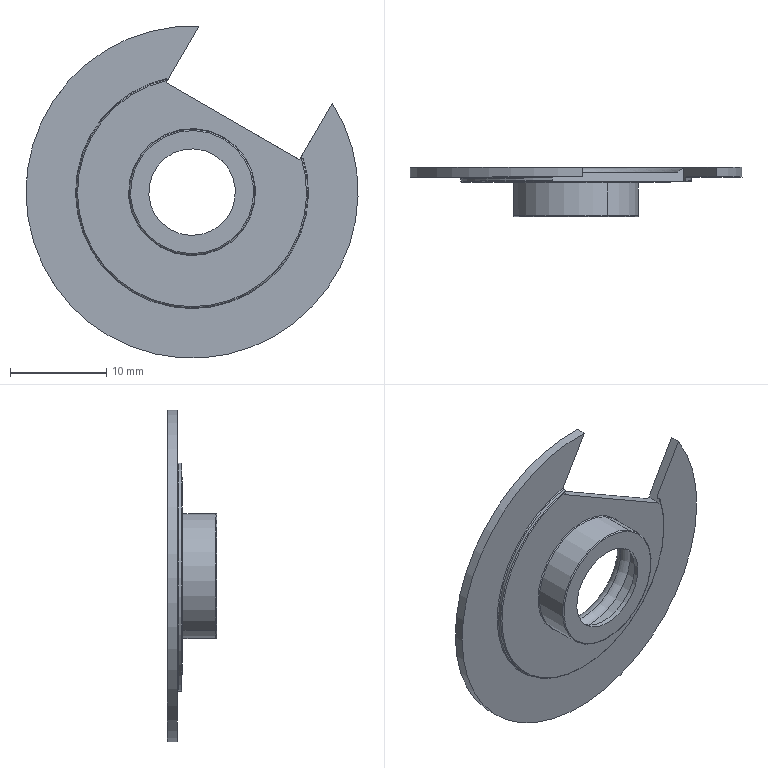Part | SolidWorks | features BaseBody 1 | 1 solid | 31 faces | box 34.501 x 5.123 x 34.5 mm | volume 825.126 mm3 | torus 14 | plane 9 | cylinder 8 | commonest cylinder face diameters 9 x2 12 x2 13 x2 24 x1 34.5 x1
STEP:
#1=CARTESIAN_POINT('',(344.717,378.167,111.682));
#2=VERTEX_POINT('',#1);
#3=CARTESIAN_POINT('',(345.266,379.267,112.635));
#4=VERTEX_POINT('',#3);
#5=CARTESIAN_POINT('',(345.267,378.167,112.635));
#6=DIRECTION('',(0.866,0.0008313,-0.5));
#7=DIRECTION('',(-0.5,0.,-0.866));
#8=AXIS2_PLACEMENT_3D('',#5,#6,#7);
#9=CIRCLE('',#8,1.1);
#10=EDGE_CURVE('',#2,#4,#9,.T.);
#11=ORIENTED_EDGE('',*,*,#10,.F.);
#12=CARTESIAN_POINT('',(339.217,378.161,102.156));
#13=VERTEX_POINT('',#12);
#14=CARTESIAN_POINT('',(341.967,378.164,106.919));
#15=DIRECTION('',(0.0009599,-1.,0.));
#16=DIRECTION('',(1.,0.0009599,0.));
#17=AXIS2_PLACEMENT_3D('',#14,#15,#16);
#18=CIRCLE('',#17,5.5);
#19=EDGE_CURVE('',#2,#13,#18,.T.);
#20=ORIENTED_EDGE('',*,*,#19,.T.);
#21=CARTESIAN_POINT('',(338.666,379.261,101.203));
#22=VERTEX_POINT('',#21);
#23=CARTESIAN_POINT('',(338.667,378.161,101.203));
#24=DIRECTION('',(-0.866,-0.0008313,0.5));
#25=DIRECTION('',(0.5,0.,0.866));
#26=AXIS2_PLACEMENT_3D('',#23,#24,#25);
#27=CIRCLE('',#26,1.1);
#28=EDGE_CURVE('',#13,#22,#27,.T.);
#29=ORIENTED_EDGE('',*,*,#28,.T.);
#30=CARTESIAN_POINT('',(341.966,379.264,106.919));
#31=DIRECTION('',(0.0009599,-1.,0.));
#32=DIRECTION('',(-0.5,-0.0004799,-0.866));
#33=AXIS2_PLACEMENT_3D('',#30,#31,#32);
#34=CIRCLE('',#33,6.6);
#35=EDGE_CURVE('',#4,#22,#34,.T.);
#36=ORIENTED_EDGE('',*,*,#35,.F.);
#37=EDGE_LOOP('',(#11,#20,#29,#36));
#38=FACE_OUTER_BOUND('',#37,.T.);
#39=CARTESIAN_POINT('',(341.967,378.164,106.919));
#40=DIRECTION('',(0.0009599,-1.,0.));
#41=DIRECTION('',(-0.5,-0.0004799,-0.866));
#42=AXIS2_PLACEMENT_3D('',#39,#40,#41);
#43=TOROIDAL_SURFACE('',#42,6.6,1.1);
#44=ADVANCED_FACE('',(#38),#43,.T.);
#45=ORIENTED_EDGE('',*,*,#28,.F.);
#46=CARTESIAN_POINT('',(341.967,378.164,106.919));
#47=DIRECTION('',(0.0009599,-1.,0.));
#48=DIRECTION('',(1.,0.0009599,0.));
#49=AXIS2_PLACEMENT_3D('',#46,#47,#48);
#50=CIRCLE('',#49,5.5);
#51=EDGE_CURVE('',#13,#2,#50,.T.);
#52=ORIENTED_EDGE('',*,*,#51,.T.);
#53=ORIENTED_EDGE('',*,*,#10,.T.);
#54=CARTESIAN_POINT('',(341.966,379.264,106.919));
#55=DIRECTION('',(0.0009599,-1.,0.));
#56=DIRECTION('',(-0.5,-0.0004799,-0.866));
#57=AXIS2_PLACEMENT_3D('',#54,#55,#56);
#58=CIRCLE('',#57,6.6);
#59=EDGE_CURVE('',#22,#4,#58,.T.);
#60=ORIENTED_EDGE('',*,*,#59,.F.);
#61=EDGE_LOOP('',(#45,#52,#53,#60));
#62=FACE_OUTER_BOUND('',#61,.T.);
#63=CARTESIAN_POINT('',(341.967,378.164,106.919));
#64=DIRECTION('',(0.0009599,-1.,0.));
#65=DIRECTION('',(-0.5,-0.0004799,-0.866));
#66=AXIS2_PLACEMENT_3D('',#63,#64,#65);
#67=TOROIDAL_SURFACE('',#66,6.6,1.1);
#68=ADVANCED_FACE('',(#62),#67,.T.);
#69=CARTESIAN_POINT('',(338.717,378.161,101.29));
#70=VERTEX_POINT('',#69);
#71=CARTESIAN_POINT('',(345.217,378.167,112.548));
#72=VERTEX_POINT('',#71);
#73=CARTESIAN_POINT('',(341.967,378.164,106.919));
#74=DIRECTION('',(-0.0009599,1.,0.));
#75=DIRECTION('',(-0.5,-0.0004799,-0.866));
#76=AXIS2_PLACEMENT_3D('',#73,#74,#75);
#77=CIRCLE('',#76,6.5);
#78=EDGE_CURVE('',#70,#72,#77,.T.);
#79=ORIENTED_EDGE('',*,*,#78,.T.);
#80=CARTESIAN_POINT('',(345.267,378.267,112.635));
#81=VERTEX_POINT('',#80);
#82=CARTESIAN_POINT('',(345.267,378.167,112.635));
#83=DIRECTION('',(0.866,0.0008313,-0.5));
#84=DIRECTION('',(-0.5,0.,-0.866));
#85=AXIS2_PLACEMENT_3D('',#82,#83,#84);
#86=CIRCLE('',#85,0.1);
#87=EDGE_CURVE('',#72,#81,#86,.T.);
#88=ORIENTED_EDGE('',*,*,#87,.T.);
#89=CARTESIAN_POINT('',(338.667,378.261,101.203));
#90=VERTEX_POINT('',#89);
#91=CARTESIAN_POINT('',(341.967,378.264,106.919));
#92=DIRECTION('',(-0.0009599,1.,0.));
#93=DIRECTION('',(0.5,0.0004799,0.866));
#94=AXIS2_PLACEMENT_3D('',#91,#92,#93);
#95=CIRCLE('',#94,6.6);
#96=EDGE_CURVE('',#90,#81,#95,.T.);
#97=ORIENTED_EDGE('',*,*,#96,.F.);
#98=CARTESIAN_POINT('',(338.667,378.161,101.203));
#99=DIRECTION('',(-0.866,-0.0008313,0.5));
#100=DIRECTION('',(0.5,0.,0.866));
#101=AXIS2_PLACEMENT_3D('',#98,#99,#100);
#102=CIRCLE('',#101,0.1);
#103=EDGE_CURVE('',#70,#90,#102,.T.);
#104=ORIENTED_EDGE('',*,*,#103,.F.);
#105=EDGE_LOOP('',(#79,#88,#97,#104));
#106=FACE_OUTER_BOUND('',#105,.T.);
#107=CARTESIAN_POINT('',(341.967,378.164,106.919));
#108=DIRECTION('',(0.0009599,-1.,0.));
#109=DIRECTION('',(-0.5,-0.0004799,-0.866));
#110=AXIS2_PLACEMENT_3D('',#107,#108,#109);
#111=TOROIDAL_SURFACE('',#110,6.6,0.1);
#112=ADVANCED_FACE('',(#106),#111,.F.);
#113=CARTESIAN_POINT('',(338.72,374.761,101.29));
#114=VERTEX_POINT('',#113);
#115=CARTESIAN_POINT('',(345.22,374.767,112.548));
#116=VERTEX_POINT('',#115);
#117=CARTESIAN_POINT('',(341.97,374.764,106.919));
#118=DIRECTION('',(0.0009599,-1.,0.));
#119=DIRECTION('',(0.5,0.0004799,0.866));
#120=AXIS2_PLACEMENT_3D('',#117,#118,#119);
#121=CIRCLE('',#120,6.5);
#122=EDGE_CURVE('',#114,#116,#121,.T.);
#123=ORIENTED_EDGE('',*,*,#122,.F.);
#124=CARTESIAN_POINT('',(338.72,374.661,101.29));
#125=DIRECTION('',(-0.0009599,1.,0.));
#126=VECTOR('',#125,1000.);
#127=LINE('',#124,#126);
#128=EDGE_CURVE('',#114,#70,#127,.T.);
#129=ORIENTED_EDGE('',*,*,#128,.T.);
#130=CARTESIAN_POINT('',(341.967,378.164,106.919));
#131=DIRECTION('',(-0.0009599,1.,0.));
#132=DIRECTION('',(-0.5,-0.0004799,-0.866));
#133=AXIS2_PLACEMENT_3D('',#130,#131,#132);
#134=CIRCLE('',#133,6.5);
#135=EDGE_CURVE('',#72,#70,#134,.T.);
#136=ORIENTED_EDGE('',*,*,#135,.F.);
#137=CARTESIAN_POINT('',(345.22,374.667,112.548));
#138=DIRECTION('',(-0.0009599,1.,0.));
#139=VECTOR('',#138,1000.);
#140=LINE('',#137,#139);
#141=EDGE_CURVE('',#116,#72,#140,.T.);
#142=ORIENTED_EDGE('',*,*,#141,.F.);
#143=EDGE_LOOP('',(#123,#129,#136,#142));
#144=FACE_OUTER_BOUND('',#143,.T.);
#145=CARTESIAN_POINT('',(341.97,374.664,106.919));
#146=DIRECTION('',(-0.0009599,1.,0.));
#147=DIRECTION('',(0.5,0.0004799,0.866));
#148=AXIS2_PLACEMENT_3D('',#145,#146,#147);
#149=CYLINDRICAL_SURFACE('',#148,6.5);
#150=ADVANCED_FACE('',(#144),#149,.T.);
#151=ORIENTED_EDGE('',*,*,#122,.T.);
#152=CARTESIAN_POINT('',(345.17,374.667,112.462));
#153=VERTEX_POINT('',#152);
#154=CARTESIAN_POINT('',(345.17,374.767,112.462));
#155=DIRECTION('',(0.866,0.0008313,-0.5));
#156=DIRECTION('',(-0.5,0.,-0.866));
#157=AXIS2_PLACEMENT_3D('',#154,#155,#156);
#158=CIRCLE('',#157,0.1);
#159=EDGE_CURVE('',#116,#153,#158,.T.);
#160=ORIENTED_EDGE('',*,*,#159,.T.);
#161=CARTESIAN_POINT('',(338.77,374.661,101.377));
#162=VERTEX_POINT('',#161);
#163=CARTESIAN_POINT('',(341.97,374.664,106.919));
#164=DIRECTION('',(0.0009599,-1.,0.));
#165=DIRECTION('',(-0.5,-0.0004799,-0.866));
#166=AXIS2_PLACEMENT_3D('',#163,#164,#165);
#167=CIRCLE('',#166,6.4);
#168=EDGE_CURVE('',#162,#153,#167,.T.);
#169=ORIENTED_EDGE('',*,*,#168,.F.);
#170=CARTESIAN_POINT('',(338.77,374.761,101.377));
#171=DIRECTION('',(-0.866,-0.0008313,0.5));
#172=DIRECTION('',(0.5,0.,0.866));
#173=AXIS2_PLACEMENT_3D('',#170,#171,#172);
#174=CIRCLE('',#173,0.1);
#175=EDGE_CURVE('',#114,#162,#174,.T.);
#176=ORIENTED_EDGE('',*,*,#175,.F.);
#177=EDGE_LOOP('',(#151,#160,#169,#176));
#178=FACE_OUTER_BOUND('',#177,.T.);
#179=CARTESIAN_POINT('',(341.97,374.764,106.919));
#180=DIRECTION('',(0.0009599,-1.,0.));
#181=DIRECTION('',(-0.5,-0.0004799,-0.866));
#182=AXIS2_PLACEMENT_3D('',#179,#180,#181);
#183=TOROIDAL_SURFACE('',#182,6.4,0.1);
#184=ADVANCED_FACE('',(#178),#183,.T.);
#185=CARTESIAN_POINT('',(344.22,375.166,110.816));
#186=VERTEX_POINT('',#185);
#187=CARTESIAN_POINT('',(339.72,375.162,103.022));
#188=VERTEX_POINT('',#187);
#189=CARTESIAN_POINT('',(341.97,375.164,106.919));
#190=DIRECTION('',(0.0009599,-1.,0.));
#191=DIRECTION('',(-0.5,-0.0004799,-0.866));
#192=AXIS2_PLACEMENT_3D('',#189,#190,#191);
#193=CIRCLE('',#192,4.5);
#194=EDGE_CURVE('',#186,#188,#193,.T.);
#195=ORIENTED_EDGE('',*,*,#194,.F.);
#196=CARTESIAN_POINT('',(344.22,374.666,110.816));
#197=VERTEX_POINT('',#196);
#198=CARTESIAN_POINT('',(344.217,378.266,110.816));
#199=DIRECTION('',(0.0009599,-1.,0.));
#200=VECTOR('',#199,1000.);
#201=LINE('',#198,#200);
#202=EDGE_CURVE('',#186,#197,#201,.T.);
#203=ORIENTED_EDGE('',*,*,#202,.T.);
#204=CARTESIAN_POINT('',(339.72,374.662,103.022));
#205=VERTEX_POINT('',#204);
#206=CARTESIAN_POINT('',(341.97,374.664,106.919));
#207=DIRECTION('',(-0.0009599,1.,0.));
#208=DIRECTION('',(-0.5,-0.0004799,-0.866));
#209=AXIS2_PLACEMENT_3D('',#206,#207,#208);
#210=CIRCLE('',#209,4.5);
#211=EDGE_CURVE('',#205,#197,#210,.T.);
#212=ORIENTED_EDGE('',*,*,#211,.F.);
#213=CARTESIAN_POINT('',(339.717,378.262,103.022));
#214=DIRECTION('',(0.0009599,-1.,0.));
#215=VECTOR('',#214,1000.);
#216=LINE('',#213,#215);
#217=EDGE_CURVE('',#188,#205,#216,.T.);
#218=ORIENTED_EDGE('',*,*,#217,.F.);
#219=EDGE_LOOP('',(#195,#203,#212,#218));
#220=FACE_OUTER_BOUND('',#219,.T.);
#221=CARTESIAN_POINT('',(341.967,378.264,106.919));
#222=DIRECTION('',(0.0009599,-1.,0.));
#223=DIRECTION('',(-0.5,-0.0004799,-0.866));
#224=AXIS2_PLACEMENT_3D('',#221,#222,#223);
#225=CYLINDRICAL_SURFACE('',#224,4.5);
#226=ADVANCED_FACE('',(#220),#225,.F.);
#227=CARTESIAN_POINT('',(338.97,375.161,101.723));
#228=VERTEX_POINT('',#227);
#229=CARTESIAN_POINT('',(344.97,375.167,112.115));
#230=VERTEX_POINT('',#229);
#231=CARTESIAN_POINT('',(341.97,375.164,106.919));
#232=DIRECTION('',(-0.0009599,1.,0.));
#233=DIRECTION('',(0.5,0.0004799,0.866));
#234=AXIS2_PLACEMENT_3D('',#231,#232,#233);
#235=CIRCLE('',#234,6.);
#236=EDGE_CURVE('',#228,#230,#235,.T.);
#237=ORIENTED_EDGE('',*,*,#236,.F.);
#238=CARTESIAN_POINT('',(338.968,377.239,101.723));
#239=VERTEX_POINT('',#238);
#240=CARTESIAN_POINT('',(338.97,374.661,101.723));
#241=DIRECTION('',(-0.0009599,1.,0.));
#242=VECTOR('',#241,1000.);
#243=LINE('',#240,#242);
#244=EDGE_CURVE('',#228,#239,#243,.T.);
#245=ORIENTED_EDGE('',*,*,#244,.T.);
#246=CARTESIAN_POINT('',(344.968,377.245,112.115));
#247=VERTEX_POINT('',#246);
#248=CARTESIAN_POINT('',(341.968,377.242,106.919));
#249=DIRECTION('',(0.0009599,-1.,0.));
#250=DIRECTION('',(0.5,0.0004799,0.866));
#251=AXIS2_PLACEMENT_3D('',#248,#249,#250);
#252=CIRCLE('',#251,6.);
#253=EDGE_CURVE('',#247,#239,#252,.T.);
#254=ORIENTED_EDGE('',*,*,#253,.F.);
#255=CARTESIAN_POINT('',(344.97,374.667,112.115));
#256=DIRECTION('',(-0.0009599,1.,0.));
#257=VECTOR('',#256,1000.);
#258=LINE('',#255,#257);
#259=EDGE_CURVE('',#230,#247,#258,.T.);
#260=ORIENTED_EDGE('',*,*,#259,.F.);
#261=EDGE_LOOP('',(#237,#245,#254,#260));
#262=FACE_OUTER_BOUND('',#261,.T.);
#263=CARTESIAN_POINT('',(341.97,374.664,106.919));
#264=DIRECTION('',(-0.0009599,1.,0.));
#265=DIRECTION('',(0.5,0.0004799,0.866));
#266=AXIS2_PLACEMENT_3D('',#263,#264,#265);
#267=CYLINDRICAL_SURFACE('',#266,6.);
#268=ADVANCED_FACE('',(#262),#267,.F.);
#269=ORIENTED_EDGE('',*,*,#51,.F.);
#270=CARTESIAN_POINT('',(338.667,378.161,101.203));
#271=DIRECTION('',(-0.866,-0.0008313,0.5));
#272=DIRECTION('',(0.5,0.,0.866));
#273=AXIS2_PLACEMENT_3D('',#270,#271,#272);
#274=CIRCLE('',#273,1.1);
#275=EDGE_CURVE('',#239,#13,#274,.T.);
#276=ORIENTED_EDGE('',*,*,#275,.F.);
#277=CARTESIAN_POINT('',(341.968,377.242,106.919));
#278=DIRECTION('',(0.0009599,-1.,0.));
#279=DIRECTION('',(0.5,0.0004799,0.866));
#280=AXIS2_PLACEMENT_3D('',#277,#278,#279);
#281=CIRCLE('',#280,6.);
#282=EDGE_CURVE('',#239,#247,#281,.T.);
#283=ORIENTED_EDGE('',*,*,#282,.T.);
#284=CARTESIAN_POINT('',(345.267,378.167,112.635));
#285=DIRECTION('',(0.866,0.0008313,-0.5));
#286=DIRECTION('',(-0.5,0.,-0.866));
#287=AXIS2_PLACEMENT_3D('',#284,#285,#286);
#288=CIRCLE('',#287,1.1);
#289=EDGE_CURVE('',#247,#2,#288,.T.);
#290=ORIENTED_EDGE('',*,*,#289,.T.);
#291=EDGE_LOOP('',(#269,#276,#283,#290));
#292=FACE_OUTER_BOUND('',#291,.T.);
#293=CARTESIAN_POINT('',(341.967,378.164,106.919));
#294=DIRECTION('',(0.0009599,-1.,0.));
#295=DIRECTION('',(-0.5,-0.0004799,-0.866));
#296=AXIS2_PLACEMENT_3D('',#293,#294,#295);
#297=TOROIDAL_SURFACE('',#296,6.6,1.1);
#298=ADVANCED_FACE('',(#292),#297,.T.);
#299=CARTESIAN_POINT('',(336.377,379.259,97.239));
#300=VERTEX_POINT('',#299);
#301=CARTESIAN_POINT('',(339.929,379.262,117.91));
#302=VERTEX_POINT('',#301);
#303=CARTESIAN_POINT('',(341.966,379.264,106.919));
#304=DIRECTION('',(-0.0009599,1.,0.));
#305=DIRECTION('',(0.9426,0.0009048,0.3338));
#306=AXIS2_PLACEMENT_3D('',#303,#304,#305);
#307=CIRCLE('',#306,11.178);
#308=EDGE_CURVE('',#300,#302,#307,.T.);
#309=ORIENTED_EDGE('',*,*,#308,.F.);
#310=CARTESIAN_POINT('',(335.915,379.758,96.44));
#311=VERTEX_POINT('',#310);
#312=CARTESIAN_POINT('',(335.916,378.658,96.44));
#313=DIRECTION('',(-0.866,-0.0008313,0.5));
#314=DIRECTION('',(0.5,0.,0.866));
#315=AXIS2_PLACEMENT_3D('',#312,#313,#314);
#316=CIRCLE('',#315,1.1);
#317=EDGE_CURVE('',#300,#311,#316,.T.);
#318=ORIENTED_EDGE('',*,*,#317,.T.);
#319=CARTESIAN_POINT('',(339.576,379.762,118.781));
#320=VERTEX_POINT('',#319);
#321=CARTESIAN_POINT('',(341.965,379.764,106.919));
#322=DIRECTION('',(0.0009599,-1.,0.));
#323=DIRECTION('',(-0.1975,-0.0001895,0.9803));
#324=AXIS2_PLACEMENT_3D('',#321,#322,#323);
#325=CIRCLE('',#324,12.1);
#326=EDGE_CURVE('',#320,#311,#325,.T.);
#327=ORIENTED_EDGE('',*,*,#326,.F.);
#328=CARTESIAN_POINT('',(339.287,379.675,118.28));
#329=VERTEX_POINT('',#328);
#330=CARTESIAN_POINT('',(339.576,379.762,118.781));
#331=CARTESIAN_POINT('',(339.478,379.762,118.61));
#332=CARTESIAN_POINT('',(339.381,379.733,118.443));
#333=CARTESIAN_POINT('',(339.287,379.675,118.28));
#334=B_SPLINE_CURVE_WITH_KNOTS('',3,(#330,#331,#332,#333),.UNSPECIFIED.,.F.,.F.,(4,4),(0.,0.0005844),.UNSPECIFIED.);
#335=EDGE_CURVE('',#320,#329,#334,.T.);
#336=ORIENTED_EDGE('',*,*,#335,.T.);
#337=CARTESIAN_POINT('',(339.287,379.675,118.28));
#338=CARTESIAN_POINT('',(339.407,379.635,118.211));
#339=CARTESIAN_POINT('',(339.521,379.583,118.145));
#340=CARTESIAN_POINT('',(339.738,379.447,118.02));
#341=CARTESIAN_POINT('',(339.841,379.364,117.961));
#342=CARTESIAN_POINT('',(339.929,379.262,117.91));
#343=B_SPLINE_CURVE_WITH_KNOTS('',3,(#337,#338,#339,#340,#341,#342),.UNSPECIFIED.,.F.,.F.,(4,2,4),(0.,0.0004263,0.0008525),.UNSPECIFIED.);
#344=EDGE_CURVE('',#329,#302,#343,.T.);
#345=ORIENTED_EDGE('',*,*,#344,.T.);
#346=EDGE_LOOP('',(#309,#318,#327,#336,#345));
#347=FACE_OUTER_BOUND('',#346,.T.);
#348=CARTESIAN_POINT('',(341.966,378.664,106.919));
#349=DIRECTION('',(0.0009599,-1.,0.));
#350=DIRECTION('',(-0.5,-0.0004799,-0.866));
#351=AXIS2_PLACEMENT_3D('',#348,#349,#350);
#352=TOROIDAL_SURFACE('',#351,12.1,1.1);
#353=ADVANCED_FACE('',(#347),#352,.T.);
#354=CARTESIAN_POINT('',(353.367,378.675,110.665));
#355=VERTEX_POINT('',#354);
#356=CARTESIAN_POINT('',(335.966,378.658,96.527));
#357=VERTEX_POINT('',#356);
#358=CARTESIAN_POINT('',(341.966,378.664,106.919));
#359=DIRECTION('',(-0.0009599,1.,0.));
#360=DIRECTION('',(0.95,0.0009119,0.3122));
#361=AXIS2_PLACEMENT_3D('',#358,#359,#360);
#362=CIRCLE('',#361,12.);
#363=EDGE_CURVE('',#355,#357,#362,.T.);
#364=ORIENTED_EDGE('',*,*,#363,.T.);
#365=CARTESIAN_POINT('',(335.916,378.758,96.44));
#366=VERTEX_POINT('',#365);
#367=CARTESIAN_POINT('',(335.916,378.658,96.44));
#368=DIRECTION('',(-0.866,-0.0008313,0.5));
#369=DIRECTION('',(0.5,0.,0.866));
#370=AXIS2_PLACEMENT_3D('',#367,#368,#369);
#371=CIRCLE('',#370,0.1);
#372=EDGE_CURVE('',#357,#366,#371,.T.);
#373=ORIENTED_EDGE('',*,*,#372,.T.);
#374=CARTESIAN_POINT('',(353.434,378.775,110.781));
#375=VERTEX_POINT('',#374);
#376=CARTESIAN_POINT('',(341.966,378.764,106.919));
#377=DIRECTION('',(-0.0009599,1.,0.));
#378=DIRECTION('',(0.9477,0.0009097,0.3192));
#379=AXIS2_PLACEMENT_3D('',#376,#377,#378);
#380=CIRCLE('',#379,12.1);
#381=EDGE_CURVE('',#375,#366,#380,.T.);
#382=ORIENTED_EDGE('',*,*,#381,.F.);
#383=CARTESIAN_POINT('',(353.367,378.675,110.665));
#384=CARTESIAN_POINT('',(353.367,378.681,110.665));
#385=CARTESIAN_POINT('',(353.367,378.693,110.666));
#386=CARTESIAN_POINT('',(353.371,378.71,110.672));
#387=CARTESIAN_POINT('',(353.376,378.727,110.681));
#388=CARTESIAN_POINT('',(353.383,378.742,110.694));
#389=CARTESIAN_POINT('',(353.393,378.755,110.71));
#390=CARTESIAN_POINT('',(353.404,378.765,110.73));
#391=CARTESIAN_POINT('',(353.418,378.773,110.753));
#392=CARTESIAN_POINT('',(353.428,378.775,110.771));
#393=CARTESIAN_POINT('',(353.434,378.775,110.781));
#394=B_SPLINE_CURVE_WITH_KNOTS('',3,(#383,#384,#385,#386,#387,#388,#389,#390,#391,#392,#393),.UNSPECIFIED.,.F.,.F.,(4,1,1,1,1,1,1,1,4),(0.,0.125,0.25,0.375,0.5,0.625,0.75,0.875,1.),.UNSPECIFIED.);
#395=EDGE_CURVE('',#355,#375,#394,.T.);
#396=ORIENTED_EDGE('',*,*,#395,.F.);
#397=EDGE_LOOP('',(#364,#373,#382,#396));
#398=FACE_OUTER_BOUND('',#397,.T.);
#399=CARTESIAN_POINT('',(341.966,378.664,106.919));
#400=DIRECTION('',(0.0009599,-1.,0.));
#401=DIRECTION('',(-0.5,-0.0004799,-0.866));
#402=AXIS2_PLACEMENT_3D('',#399,#400,#401);
#403=TOROIDAL_SURFACE('',#402,12.1,0.1);
#404=ADVANCED_FACE('',(#398),#403,.F.);
#405=CARTESIAN_POINT('',(339.511,378.362,118.665));
#406=VERTEX_POINT('',#405);
#407=CARTESIAN_POINT('',(335.967,378.358,96.527));
#408=VERTEX_POINT('',#407);
#409=CARTESIAN_POINT('',(341.967,378.364,106.919));
#410=DIRECTION('',(0.0009599,-1.,0.));
#411=DIRECTION('',(-0.5,-0.0004799,-0.866));
#412=AXIS2_PLACEMENT_3D('',#409,#410,#411);
#413=CIRCLE('',#412,12.);
#414=EDGE_CURVE('',#406,#408,#413,.T.);
#415=ORIENTED_EDGE('',*,*,#414,.T.);
#416=CARTESIAN_POINT('',(336.017,378.258,96.613));
#417=VERTEX_POINT('',#416);
#418=CARTESIAN_POINT('',(336.017,378.358,96.613));
#419=DIRECTION('',(-0.866,-0.0008313,0.5));
#420=DIRECTION('',(0.5,0.,0.866));
#421=AXIS2_PLACEMENT_3D('',#418,#419,#420);
#422=CIRCLE('',#421,0.1);
#423=EDGE_CURVE('',#408,#417,#422,.T.);
#424=ORIENTED_EDGE('',*,*,#423,.T.);
#425=CARTESIAN_POINT('',(339.443,378.262,118.549));
#426=VERTEX_POINT('',#425);
#427=CARTESIAN_POINT('',(341.967,378.264,106.919));
#428=DIRECTION('',(0.0009599,-1.,0.));
#429=DIRECTION('',(-0.212,-0.0002035,0.9773));
#430=AXIS2_PLACEMENT_3D('',#427,#428,#429);
#431=CIRCLE('',#430,11.9);
#432=EDGE_CURVE('',#426,#417,#431,.T.);
#433=ORIENTED_EDGE('',*,*,#432,.F.);
#434=CARTESIAN_POINT('',(339.443,378.262,118.549));
#435=CARTESIAN_POINT('',(339.45,378.262,118.559));
#436=CARTESIAN_POINT('',(339.462,378.264,118.58));
#437=CARTESIAN_POINT('',(339.477,378.274,118.607));
#438=CARTESIAN_POINT('',(339.49,378.288,118.629));
#439=CARTESIAN_POINT('',(339.5,378.305,118.646));
#440=CARTESIAN_POINT('',(339.506,378.323,118.657));
#441=CARTESIAN_POINT('',(339.51,378.342,118.664));
#442=CARTESIAN_POINT('',(339.511,378.355,118.665));
#443=CARTESIAN_POINT('',(339.511,378.362,118.665));
#444=B_SPLINE_CURVE_WITH_KNOTS('',3,(#434,#435,#436,#437,#438,#439,#440,#441,#442,#443),.UNSPECIFIED.,.F.,.F.,(4,1,1,1,1,1,1,4),(0.,0.1429,0.2857,0.4286,0.5714,0.7143,0.8571,1.),.UNSPECIFIED.);
#445=EDGE_CURVE('',#426,#406,#444,.T.);
#446=ORIENTED_EDGE('',*,*,#445,.T.);
#447=EDGE_LOOP('',(#415,#424,#433,#446));
#448=FACE_OUTER_BOUND('',#447,.T.);
#449=CARTESIAN_POINT('',(341.967,378.364,106.919));
#450=DIRECTION('',(0.0009599,-1.,0.));
#451=DIRECTION('',(-0.5,-0.0004799,-0.866));
#452=AXIS2_PLACEMENT_3D('',#449,#450,#451);
#453=TOROIDAL_SURFACE('',#452,11.9,0.1);
#454=ADVANCED_FACE('',(#448),#453,.T.);
#455=ORIENTED_EDGE('',*,*,#423,.F.);
#456=CARTESIAN_POINT('',(353.367,378.375,110.665));
#457=VERTEX_POINT('',#456);
#458=CARTESIAN_POINT('',(341.967,378.364,106.919));
#459=DIRECTION('',(0.0009599,-1.,0.));
#460=DIRECTION('',(-0.5,-0.0004799,-0.866));
#461=AXIS2_PLACEMENT_3D('',#458,#459,#460);
#462=CIRCLE('',#461,12.);
#463=EDGE_CURVE('',#408,#457,#462,.T.);
#464=ORIENTED_EDGE('',*,*,#463,.T.);
#465=CARTESIAN_POINT('',(353.3,378.275,110.549));
#466=VERTEX_POINT('',#465);
#467=CARTESIAN_POINT('',(353.367,378.375,110.665));
#468=CARTESIAN_POINT('',(353.367,378.369,110.665));
#469=CARTESIAN_POINT('',(353.366,378.356,110.664));
#470=CARTESIAN_POINT('',(353.363,378.337,110.657));
#471=CARTESIAN_POINT('',(353.356,378.318,110.646));
#472=CARTESIAN_POINT('',(353.346,378.301,110.629));
#473=CARTESIAN_POINT('',(353.334,378.287,110.607));
#474=CARTESIAN_POINT('',(353.318,378.277,110.58));
#475=CARTESIAN_POINT('',(353.306,378.275,110.559));
#476=CARTESIAN_POINT('',(353.3,378.275,110.549));
#477=B_SPLINE_CURVE_WITH_KNOTS('',3,(#467,#468,#469,#470,#471,#472,#473,#474,#475,#476),.UNSPECIFIED.,.F.,.F.,(4,1,1,1,1,1,1,4),(0.,0.1429,0.2857,0.4286,0.5714,0.7143,0.8571,1.),.UNSPECIFIED.);
#478=EDGE_CURVE('',#457,#466,#477,.T.);
#479=ORIENTED_EDGE('',*,*,#478,.T.);
#480=CARTESIAN_POINT('',(341.967,378.264,106.919));
#481=DIRECTION('',(0.0009599,-1.,0.));
#482=DIRECTION('',(-0.212,-0.0002035,0.9773));
#483=AXIS2_PLACEMENT_3D('',#480,#481,#482);
#484=CIRCLE('',#483,11.9);
#485=EDGE_CURVE('',#417,#466,#484,.T.);
#486=ORIENTED_EDGE('',*,*,#485,.F.);
#487=EDGE_LOOP('',(#455,#464,#479,#486));
#488=FACE_OUTER_BOUND('',#487,.T.);
#489=CARTESIAN_POINT('',(341.967,378.364,106.919));
#490=DIRECTION('',(0.0009599,-1.,0.));
#491=DIRECTION('',(-0.5,-0.0004799,-0.866));
#492=AXIS2_PLACEMENT_3D('',#489,#490,#491);
#493=TOROIDAL_SURFACE('',#492,11.9,0.1);
#494=ADVANCED_FACE('',(#488),#493,.T.);
#495=ORIENTED_EDGE('',*,*,#363,.F.);
#496=CARTESIAN_POINT('',(353.367,378.675,110.665));
#497=DIRECTION('',(0.0009599,-1.,0.));
#498=VECTOR('',#497,1000.);
#499=LINE('',#496,#498);
#500=EDGE_CURVE('',#355,#457,#499,.T.);
#501=ORIENTED_EDGE('',*,*,#500,.T.);
#502=ORIENTED_EDGE('',*,*,#463,.F.);
#503=ORIENTED_EDGE('',*,*,#414,.F.);
#504=CARTESIAN_POINT('',(339.51,378.662,118.665));
#505=VERTEX_POINT('',#504);
#506=CARTESIAN_POINT('',(339.511,378.362,118.665));
#507=DIRECTION('',(-0.0009599,1.,0.));
#508=VECTOR('',#507,1000.);
#509=LINE('',#506,#508);
#510=EDGE_CURVE('',#406,#505,#509,.T.);
#511=ORIENTED_EDGE('',*,*,#510,.T.);
#512=CARTESIAN_POINT('',(341.966,378.664,106.919));
#513=DIRECTION('',(-0.0009599,1.,0.));
#514=DIRECTION('',(0.95,0.0009119,0.3122));
#515=AXIS2_PLACEMENT_3D('',#512,#513,#514);
#516=CIRCLE('',#515,12.);
#517=EDGE_CURVE('',#357,#505,#516,.T.);
#518=ORIENTED_EDGE('',*,*,#517,.F.);
#519=EDGE_LOOP('',(#495,#501,#502,#503,#511,#518));
#520=FACE_OUTER_BOUND('',#519,.T.);
#521=CARTESIAN_POINT('',(341.967,378.264,106.919));
#522=DIRECTION('',(-0.0009599,1.,0.));
#523=DIRECTION('',(0.5,0.0004799,0.866));
#524=AXIS2_PLACEMENT_3D('',#521,#522,#523);
#525=CYLINDRICAL_SURFACE('',#524,12.);
#526=ADVANCED_FACE('',(#520),#525,.T.);
#527=ORIENTED_EDGE('',*,*,#372,.F.);
#528=ORIENTED_EDGE('',*,*,#517,.T.);
#529=CARTESIAN_POINT('',(339.577,378.762,118.781));
#530=VERTEX_POINT('',#529);
#531=CARTESIAN_POINT('',(339.577,378.762,118.781));
#532=CARTESIAN_POINT('',(339.572,378.762,118.771));
#533=CARTESIAN_POINT('',(339.561,378.76,118.753));
#534=CARTESIAN_POINT('',(339.548,378.752,118.73));
#535=CARTESIAN_POINT('',(339.536,378.741,118.71));
#536=CARTESIAN_POINT('',(339.527,378.728,118.694));
#537=CARTESIAN_POINT('',(339.52,378.713,118.681));
#538=CARTESIAN_POINT('',(339.514,378.697,118.672));
#539=CARTESIAN_POINT('',(339.511,378.679,118.666));
#540=CARTESIAN_POINT('',(339.51,378.668,118.665));
#541=CARTESIAN_POINT('',(339.51,378.662,118.665));
#542=B_SPLINE_CURVE_WITH_KNOTS('',3,(#531,#532,#533,#534,#535,#536,#537,#538,#539,#540,#541),.UNSPECIFIED.,.F.,.F.,(4,1,1,1,1,1,1,1,4),(0.,0.125,0.25,0.375,0.5,0.625,0.75,0.875,1.),.UNSPECIFIED.);
#543=EDGE_CURVE('',#530,#505,#542,.T.);
#544=ORIENTED_EDGE('',*,*,#543,.F.);
#545=CARTESIAN_POINT('',(341.966,378.764,106.919));
#546=DIRECTION('',(-0.0009599,1.,0.));
#547=DIRECTION('',(0.9477,0.0009097,0.3192));
#548=AXIS2_PLACEMENT_3D('',#545,#546,#547);
#549=CIRCLE('',#548,12.1);
#550=EDGE_CURVE('',#366,#530,#549,.T.);
#551=ORIENTED_EDGE('',*,*,#550,.F.);
#552=EDGE_LOOP('',(#527,#528,#544,#551));
#553=FACE_OUTER_BOUND('',#552,.T.);
#554=CARTESIAN_POINT('',(341.966,378.664,106.919));
#555=DIRECTION('',(0.0009599,-1.,0.));
#556=DIRECTION('',(-0.5,-0.0004799,-0.866));
#557=AXIS2_PLACEMENT_3D('',#554,#555,#556);
#558=TOROIDAL_SURFACE('',#557,12.1,0.1);
#559=ADVANCED_FACE('',(#553),#558,.F.);
#560=ORIENTED_EDGE('',*,*,#478,.F.);
#561=ORIENTED_EDGE('',*,*,#500,.F.);
#562=ORIENTED_EDGE('',*,*,#395,.T.);
#563=CARTESIAN_POINT('',(356.536,378.778,116.154));
#564=VERTEX_POINT('',#563);
#565=CARTESIAN_POINT('',(356.536,378.778,116.154));
#566=DIRECTION('',(-0.5,-0.0004799,-0.866));
#567=VECTOR('',#566,1000.);
#568=LINE('',#565,#567);
#569=EDGE_CURVE('',#564,#375,#568,.T.);
#570=ORIENTED_EDGE('',*,*,#569,.F.);
#571=CARTESIAN_POINT('',(356.535,379.778,116.154));
#572=VERTEX_POINT('',#571);
#573=CARTESIAN_POINT('',(356.535,379.778,116.154));
#574=DIRECTION('',(0.0009599,-1.,0.));
#575=VECTOR('',#574,1000.);
#576=LINE('',#573,#575);
#577=EDGE_CURVE('',#572,#564,#576,.T.);
#578=ORIENTED_EDGE('',*,*,#577,.F.);
#579=CARTESIAN_POINT('',(353.433,379.775,110.781));
#580=VERTEX_POINT('',#579);
#581=CARTESIAN_POINT('',(356.535,379.778,116.154));
#582=DIRECTION('',(-0.5,-0.0004799,-0.866));
#583=VECTOR('',#582,1000.);
#584=LINE('',#581,#583);
#585=EDGE_CURVE('',#572,#580,#584,.T.);
#586=ORIENTED_EDGE('',*,*,#585,.T.);
#587=CARTESIAN_POINT('',(353.144,379.688,110.28));
#588=VERTEX_POINT('',#587);
#589=CARTESIAN_POINT('',(353.144,379.688,110.28));
#590=CARTESIAN_POINT('',(353.238,379.746,110.443));
#591=CARTESIAN_POINT('',(353.334,379.775,110.61));
#592=CARTESIAN_POINT('',(353.433,379.775,110.781));
#593=B_SPLINE_CURVE_WITH_KNOTS('',3,(#589,#590,#591,#592),.UNSPECIFIED.,.F.,.F.,(4,4),(0.,0.0005844),.UNSPECIFIED.);
#594=EDGE_CURVE('',#588,#580,#593,.T.);
#595=ORIENTED_EDGE('',*,*,#594,.F.);
#596=CARTESIAN_POINT('',(353.145,378.275,110.28));
#597=VERTEX_POINT('',#596);
#598=CARTESIAN_POINT('',(353.145,378.275,110.28));
#599=DIRECTION('',(-0.0009599,1.,0.));
#600=VECTOR('',#599,1000.);
#601=LINE('',#598,#600);
#602=EDGE_CURVE('',#597,#588,#601,.T.);
#603=ORIENTED_EDGE('',*,*,#602,.F.);
#604=CARTESIAN_POINT('',(353.3,378.275,110.549));
#605=DIRECTION('',(-0.5,-0.0004799,-0.866));
#606=VECTOR('',#605,1000.);
#607=LINE('',#604,#606);
#608=EDGE_CURVE('',#466,#597,#607,.T.);
#609=ORIENTED_EDGE('',*,*,#608,.F.);
#610=EDGE_LOOP('',(#560,#561,#562,#570,#578,#586,#595,#603,#609));
#611=FACE_OUTER_BOUND('',#610,.T.);
#612=CARTESIAN_POINT('',(353.141,382.275,110.28));
#613=DIRECTION('',(0.866,0.0008313,-0.5));
#614=DIRECTION('',(0.,-1.,-0.001663));
#615=AXIS2_PLACEMENT_3D('',#612,#613,#614);
#616=PLANE('',#615);
#617=ADVANCED_FACE('',(#611),#616,.F.);
#618=ORIENTED_EDGE('',*,*,#381,.T.);
#619=ORIENTED_EDGE('',*,*,#550,.T.);
#620=CARTESIAN_POINT('',(342.68,378.765,124.154));
#621=VERTEX_POINT('',#620);
#622=CARTESIAN_POINT('',(339.577,378.762,118.781));
#623=DIRECTION('',(0.5,0.0004799,0.866));
#624=VECTOR('',#623,1000.);
#625=LINE('',#622,#624);
#626=EDGE_CURVE('',#530,#621,#625,.T.);
#627=ORIENTED_EDGE('',*,*,#626,.T.);
#628=CARTESIAN_POINT('',(341.966,378.764,106.919));
#629=DIRECTION('',(0.0009599,-1.,0.));
#630=DIRECTION('',(0.04134,0.00003968,0.9991));
#631=AXIS2_PLACEMENT_3D('',#628,#629,#630);
#632=CIRCLE('',#631,17.25);
#633=EDGE_CURVE('',#621,#564,#632,.T.);
#634=ORIENTED_EDGE('',*,*,#633,.T.);
#635=ORIENTED_EDGE('',*,*,#569,.T.);
#636=EDGE_LOOP('',(#618,#619,#627,#634,#635));
#637=FACE_OUTER_BOUND('',#636,.T.);
#638=CARTESIAN_POINT('',(341.966,378.764,106.919));
#639=DIRECTION('',(0.0009599,-1.,0.));
#640=DIRECTION('',(0.,0.,-1.));
#641=AXIS2_PLACEMENT_3D('',#638,#639,#640);
#642=PLANE('',#641);
#643=ADVANCED_FACE('',(#637),#642,.T.);
#644=ORIENTED_EDGE('',*,*,#577,.T.);
#645=ORIENTED_EDGE('',*,*,#633,.F.);
#646=CARTESIAN_POINT('',(342.679,379.765,124.154));
#647=VERTEX_POINT('',#646);
#648=CARTESIAN_POINT('',(342.68,378.765,124.154));
#649=DIRECTION('',(-0.0009599,1.,0.));
#650=VECTOR('',#649,1000.);
#651=LINE('',#648,#650);
#652=EDGE_CURVE('',#621,#647,#651,.T.);
#653=ORIENTED_EDGE('',*,*,#652,.T.);
#654=CARTESIAN_POINT('',(341.965,379.764,106.919));
#655=DIRECTION('',(-0.0009599,1.,0.));
#656=DIRECTION('',(0.8446,0.0008107,0.5354));
#657=AXIS2_PLACEMENT_3D('',#654,#655,#656);
#658=CIRCLE('',#657,17.25);
#659=EDGE_CURVE('',#572,#647,#658,.T.);
#660=ORIENTED_EDGE('',*,*,#659,.F.);
#661=EDGE_LOOP('',(#644,#645,#653,#660));
#662=FACE_OUTER_BOUND('',#661,.T.);
#663=CARTESIAN_POINT('',(341.966,378.764,106.919));
#664=DIRECTION('',(-0.0009599,1.,0.));
#665=DIRECTION('',(0.5,0.0004799,0.866));
#666=AXIS2_PLACEMENT_3D('',#663,#664,#665);
#667=CYLINDRICAL_SURFACE('',#666,17.25);
#668=ADVANCED_FACE('',(#662),#667,.T.);
#669=ORIENTED_EDGE('',*,*,#585,.F.);
#670=ORIENTED_EDGE('',*,*,#659,.T.);
#671=CARTESIAN_POINT('',(339.576,379.762,118.781));
#672=DIRECTION('',(0.5,0.0004799,0.866));
#673=VECTOR('',#672,1000.);
#674=LINE('',#671,#673);
#675=EDGE_CURVE('',#320,#647,#674,.T.);
#676=ORIENTED_EDGE('',*,*,#675,.F.);
#677=ORIENTED_EDGE('',*,*,#326,.T.);
#678=CARTESIAN_POINT('',(341.965,379.764,106.919));
#679=DIRECTION('',(0.0009599,-1.,0.));
#680=DIRECTION('',(-0.1975,-0.0001895,0.9803));
#681=AXIS2_PLACEMENT_3D('',#678,#679,#680);
#682=CIRCLE('',#681,12.1);
#683=EDGE_CURVE('',#311,#580,#682,.T.);
#684=ORIENTED_EDGE('',*,*,#683,.T.);
#685=EDGE_LOOP('',(#669,#670,#676,#677,#684));
#686=FACE_OUTER_BOUND('',#685,.T.);
#687=CARTESIAN_POINT('',(341.965,379.764,106.919));
#688=DIRECTION('',(0.0009599,-1.,0.));
#689=DIRECTION('',(0.,0.,-1.));
#690=AXIS2_PLACEMENT_3D('',#687,#688,#689);
#691=PLANE('',#690);
#692=ADVANCED_FACE('',(#686),#691,.F.);
#693=ORIENTED_EDGE('',*,*,#602,.T.);
#694=CARTESIAN_POINT('',(352.503,379.274,110.651));
#695=VERTEX_POINT('',#694);
#696=CARTESIAN_POINT('',(352.503,379.274,110.651));
#697=CARTESIAN_POINT('',(352.591,379.376,110.6));
#698=CARTESIAN_POINT('',(352.691,379.458,110.542));
#699=CARTESIAN_POINT('',(352.908,379.594,110.417));
#700=CARTESIAN_POINT('',(353.024,379.648,110.349));
#701=CARTESIAN_POINT('',(353.144,379.688,110.28));
#702=B_SPLINE_CURVE_WITH_KNOTS('',3,(#696,#697,#698,#699,#700,#701),.UNSPECIFIED.,.F.,.F.,(4,2,4),(0.,0.0004253,0.0008505),.UNSPECIFIED.);
#703=EDGE_CURVE('',#695,#588,#702,.T.);
#704=ORIENTED_EDGE('',*,*,#703,.F.);
#705=CARTESIAN_POINT('',(352.503,379.274,110.651));
#706=DIRECTION('',(-0.866,-0.0008313,0.5));
#707=VECTOR('',#706,1000.);
#708=LINE('',#705,#707);
#709=EDGE_CURVE('',#695,#302,#708,.T.);
#710=ORIENTED_EDGE('',*,*,#709,.T.);
#711=ORIENTED_EDGE('',*,*,#344,.F.);
#712=CARTESIAN_POINT('',(339.289,378.261,118.28));
#713=VERTEX_POINT('',#712);
#714=CARTESIAN_POINT('',(339.289,378.261,118.28));
#715=DIRECTION('',(-0.0009599,1.,0.));
#716=VECTOR('',#715,1000.);
#717=LINE('',#714,#716);
#718=EDGE_CURVE('',#713,#329,#717,.T.);
#719=ORIENTED_EDGE('',*,*,#718,.F.);
#720=CARTESIAN_POINT('',(353.145,378.275,110.28));
#721=DIRECTION('',(-0.866,-0.0008313,0.5));
#722=VECTOR('',#721,1000.);
#723=LINE('',#720,#722);
#724=EDGE_CURVE('',#597,#713,#723,.T.);
#725=ORIENTED_EDGE('',*,*,#724,.F.);
#726=EDGE_LOOP('',(#693,#704,#710,#711,#719,#725));
#727=FACE_OUTER_BOUND('',#726,.T.);
#728=CARTESIAN_POINT('',(339.285,382.261,118.28));
#729=DIRECTION('',(-0.5,-0.0004799,-0.866));
#730=DIRECTION('',(-0.866,0.,0.5));
#731=AXIS2_PLACEMENT_3D('',#728,#729,#730);
#732=PLANE('',#731);
#733=ADVANCED_FACE('',(#727),#732,.F.);
#734=ORIENTED_EDGE('',*,*,#317,.F.);
#735=CARTESIAN_POINT('',(341.966,379.264,106.919));
#736=DIRECTION('',(-0.0009599,1.,0.));
#737=DIRECTION('',(0.9426,0.0009048,0.3338));
#738=AXIS2_PLACEMENT_3D('',#735,#736,#737);
#739=CIRCLE('',#738,11.178);
#740=EDGE_CURVE('',#695,#300,#739,.T.);
#741=ORIENTED_EDGE('',*,*,#740,.F.);
#742=ORIENTED_EDGE('',*,*,#703,.T.);
#743=ORIENTED_EDGE('',*,*,#594,.T.);
#744=ORIENTED_EDGE('',*,*,#683,.F.);
#745=EDGE_LOOP('',(#734,#741,#742,#743,#744));
#746=FACE_OUTER_BOUND('',#745,.T.);
#747=CARTESIAN_POINT('',(341.966,378.664,106.919));
#748=DIRECTION('',(0.0009599,-1.,0.));
#749=DIRECTION('',(-0.5,-0.0004799,-0.866));
#750=AXIS2_PLACEMENT_3D('',#747,#748,#749);
#751=TOROIDAL_SURFACE('',#750,12.1,1.1);
#752=ADVANCED_FACE('',(#746),#751,.T.);
#753=ORIENTED_EDGE('',*,*,#59,.T.);
#754=ORIENTED_EDGE('',*,*,#35,.T.);
#755=EDGE_LOOP('',(#753,#754));
#756=FACE_BOUND('',#755,.T.);
#757=ORIENTED_EDGE('',*,*,#709,.F.);
#758=ORIENTED_EDGE('',*,*,#740,.T.);
#759=ORIENTED_EDGE('',*,*,#308,.T.);
#760=EDGE_LOOP('',(#757,#758,#759));
#761=FACE_OUTER_BOUND('',#760,.T.);
#762=CARTESIAN_POINT('',(341.966,379.264,106.919));
#763=DIRECTION('',(0.0009599,-1.,0.));
#764=DIRECTION('',(0.,0.,-1.));
#765=AXIS2_PLACEMENT_3D('',#762,#763,#764);
#766=PLANE('',#765);
#767=ADVANCED_FACE('',(#756,#761),#766,.F.);
#768=ORIENTED_EDGE('',*,*,#19,.F.);
#769=ORIENTED_EDGE('',*,*,#289,.F.);
#770=ORIENTED_EDGE('',*,*,#253,.T.);
#771=ORIENTED_EDGE('',*,*,#275,.T.);
#772=EDGE_LOOP('',(#768,#769,#770,#771));
#773=FACE_OUTER_BOUND('',#772,.T.);
#774=CARTESIAN_POINT('',(341.967,378.164,106.919));
#775=DIRECTION('',(0.0009599,-1.,0.));
#776=DIRECTION('',(-0.5,-0.0004799,-0.866));
#777=AXIS2_PLACEMENT_3D('',#774,#775,#776);
#778=TOROIDAL_SURFACE('',#777,6.6,1.1);
#779=ADVANCED_FACE('',(#773),#778,.T.);
#780=ORIENTED_EDGE('',*,*,#244,.F.);
#781=CARTESIAN_POINT('',(341.97,375.164,106.919));
#782=DIRECTION('',(-0.0009599,1.,0.));
#783=DIRECTION('',(0.5,0.0004799,0.866));
#784=AXIS2_PLACEMENT_3D('',#781,#782,#783);
#785=CIRCLE('',#784,6.);
#786=EDGE_CURVE('',#230,#228,#785,.T.);
#787=ORIENTED_EDGE('',*,*,#786,.F.);
#788=ORIENTED_EDGE('',*,*,#259,.T.);
#789=ORIENTED_EDGE('',*,*,#282,.F.);
#790=EDGE_LOOP('',(#780,#787,#788,#789));
#791=FACE_OUTER_BOUND('',#790,.T.);
#792=CARTESIAN_POINT('',(341.97,374.664,106.919));
#793=DIRECTION('',(-0.0009599,1.,0.));
#794=DIRECTION('',(0.5,0.0004799,0.866));
#795=AXIS2_PLACEMENT_3D('',#792,#793,#794);
#796=CYLINDRICAL_SURFACE('',#795,6.);
#797=ADVANCED_FACE('',(#791),#796,.F.);
#798=CARTESIAN_POINT('',(341.97,375.164,106.919));
#799=DIRECTION('',(0.0009599,-1.,0.));
#800=DIRECTION('',(-0.5,-0.0004799,-0.866));
#801=AXIS2_PLACEMENT_3D('',#798,#799,#800);
#802=CIRCLE('',#801,4.5);
#803=EDGE_CURVE('',#188,#186,#802,.T.);
#804=ORIENTED_EDGE('',*,*,#803,.T.);
#805=ORIENTED_EDGE('',*,*,#194,.T.);
#806=EDGE_LOOP('',(#804,#805));
#807=FACE_BOUND('',#806,.T.);
#808=ORIENTED_EDGE('',*,*,#786,.T.);
#809=ORIENTED_EDGE('',*,*,#236,.T.);
#810=EDGE_LOOP('',(#808,#809));
#811=FACE_OUTER_BOUND('',#810,.T.);
#812=CARTESIAN_POINT('',(341.97,375.164,106.919));
#813=DIRECTION('',(0.0009599,-1.,0.));
#814=DIRECTION('',(0.,0.,-1.));
#815=AXIS2_PLACEMENT_3D('',#812,#813,#814);
#816=PLANE('',#815);
#817=ADVANCED_FACE('',(#807,#811),#816,.F.);
#818=ORIENTED_EDGE('',*,*,#202,.F.);
#819=ORIENTED_EDGE('',*,*,#803,.F.);
#820=ORIENTED_EDGE('',*,*,#217,.T.);
#821=CARTESIAN_POINT('',(341.97,374.664,106.919));
#822=DIRECTION('',(-0.0009599,1.,0.));
#823=DIRECTION('',(-0.5,-0.0004799,-0.866));
#824=AXIS2_PLACEMENT_3D('',#821,#822,#823);
#825=CIRCLE('',#824,4.5);
#826=EDGE_CURVE('',#197,#205,#825,.T.);
#827=ORIENTED_EDGE('',*,*,#826,.F.);
#828=EDGE_LOOP('',(#818,#819,#820,#827));
#829=FACE_OUTER_BOUND('',#828,.T.);
#830=CARTESIAN_POINT('',(341.967,378.264,106.919));
#831=DIRECTION('',(0.0009599,-1.,0.));
#832=DIRECTION('',(-0.5,-0.0004799,-0.866));
#833=AXIS2_PLACEMENT_3D('',#830,#831,#832);
#834=CYLINDRICAL_SURFACE('',#833,4.5);
#835=ADVANCED_FACE('',(#829),#834,.F.);
#836=ORIENTED_EDGE('',*,*,#211,.T.);
#837=ORIENTED_EDGE('',*,*,#826,.T.);
#838=EDGE_LOOP('',(#836,#837));
#839=FACE_BOUND('',#838,.T.);
#840=ORIENTED_EDGE('',*,*,#168,.T.);
#841=CARTESIAN_POINT('',(341.97,374.664,106.919));
#842=DIRECTION('',(0.0009599,-1.,0.));
#843=DIRECTION('',(-0.5,-0.0004799,-0.866));
#844=AXIS2_PLACEMENT_3D('',#841,#842,#843);
#845=CIRCLE('',#844,6.4);
#846=EDGE_CURVE('',#153,#162,#845,.T.);
#847=ORIENTED_EDGE('',*,*,#846,.T.);
#848=EDGE_LOOP('',(#840,#847));
#849=FACE_OUTER_BOUND('',#848,.T.);
#850=CARTESIAN_POINT('',(341.97,374.664,106.919));
#851=DIRECTION('',(0.0009599,-1.,0.));
#852=DIRECTION('',(0.,0.,-1.));
#853=AXIS2_PLACEMENT_3D('',#850,#851,#852);
#854=PLANE('',#853);
#855=ADVANCED_FACE('',(#839,#849),#854,.T.);
#856=ORIENTED_EDGE('',*,*,#159,.F.);
#857=CARTESIAN_POINT('',(341.97,374.764,106.919));
#858=DIRECTION('',(0.0009599,-1.,0.));
#859=DIRECTION('',(0.5,0.0004799,0.866));
#860=AXIS2_PLACEMENT_3D('',#857,#858,#859);
#861=CIRCLE('',#860,6.5);
#862=EDGE_CURVE('',#116,#114,#861,.T.);
#863=ORIENTED_EDGE('',*,*,#862,.T.);
#864=ORIENTED_EDGE('',*,*,#175,.T.);
#865=ORIENTED_EDGE('',*,*,#846,.F.);
#866=EDGE_LOOP('',(#856,#863,#864,#865));
#867=FACE_OUTER_BOUND('',#866,.T.);
#868=CARTESIAN_POINT('',(341.97,374.764,106.919));
#869=DIRECTION('',(0.0009599,-1.,0.));
#870=DIRECTION('',(-0.5,-0.0004799,-0.866));
#871=AXIS2_PLACEMENT_3D('',#868,#869,#870);
#872=TOROIDAL_SURFACE('',#871,6.4,0.1);
#873=ADVANCED_FACE('',(#867),#872,.T.);
#874=ORIENTED_EDGE('',*,*,#128,.F.);
#875=ORIENTED_EDGE('',*,*,#862,.F.);
#876=ORIENTED_EDGE('',*,*,#141,.T.);
#877=ORIENTED_EDGE('',*,*,#78,.F.);
#878=EDGE_LOOP('',(#874,#875,#876,#877));
#879=FACE_OUTER_BOUND('',#878,.T.);
#880=CARTESIAN_POINT('',(341.97,374.664,106.919));
#881=DIRECTION('',(-0.0009599,1.,0.));
#882=DIRECTION('',(0.5,0.0004799,0.866));
#883=AXIS2_PLACEMENT_3D('',#880,#881,#882);
#884=CYLINDRICAL_SURFACE('',#883,6.5);
#885=ADVANCED_FACE('',(#879),#884,.T.);
#886=ORIENTED_EDGE('',*,*,#87,.F.);
#887=ORIENTED_EDGE('',*,*,#135,.T.);
#888=ORIENTED_EDGE('',*,*,#103,.T.);
#889=CARTESIAN_POINT('',(341.967,378.264,106.919));
#890=DIRECTION('',(-0.0009599,1.,0.));
#891=DIRECTION('',(0.5,0.0004799,0.866));
#892=AXIS2_PLACEMENT_3D('',#889,#890,#891);
#893=CIRCLE('',#892,6.6);
#894=EDGE_CURVE('',#81,#90,#893,.T.);
#895=ORIENTED_EDGE('',*,*,#894,.F.);
#896=EDGE_LOOP('',(#886,#887,#888,#895));
#897=FACE_OUTER_BOUND('',#896,.T.);
#898=CARTESIAN_POINT('',(341.967,378.164,106.919));
#899=DIRECTION('',(0.0009599,-1.,0.));
#900=DIRECTION('',(-0.5,-0.0004799,-0.866));
#901=AXIS2_PLACEMENT_3D('',#898,#899,#900);
#902=TOROIDAL_SURFACE('',#901,6.6,0.1);
#903=ADVANCED_FACE('',(#897),#902,.F.);
#904=ORIENTED_EDGE('',*,*,#96,.T.);
#905=ORIENTED_EDGE('',*,*,#894,.T.);
#906=EDGE_LOOP('',(#904,#905));
#907=FACE_BOUND('',#906,.T.);
#908=ORIENTED_EDGE('',*,*,#724,.T.);
#909=CARTESIAN_POINT('',(339.289,378.261,118.28));
#910=DIRECTION('',(0.5,0.0004799,0.866));
#911=VECTOR('',#910,1000.);
#912=LINE('',#909,#911);
#913=EDGE_CURVE('',#713,#426,#912,.T.);
#914=ORIENTED_EDGE('',*,*,#913,.T.);
#915=ORIENTED_EDGE('',*,*,#432,.T.);
#916=ORIENTED_EDGE('',*,*,#485,.T.);
#917=ORIENTED_EDGE('',*,*,#608,.T.);
#918=EDGE_LOOP('',(#908,#914,#915,#916,#917));
#919=FACE_OUTER_BOUND('',#918,.T.);
#920=CARTESIAN_POINT('',(341.967,378.264,106.919));
#921=DIRECTION('',(0.0009599,-1.,0.));
#922=DIRECTION('',(0.,0.,-1.));
#923=AXIS2_PLACEMENT_3D('',#920,#921,#922);
#924=PLANE('',#923);
#925=ADVANCED_FACE('',(#907,#919),#924,.T.);
#926=ORIENTED_EDGE('',*,*,#718,.T.);
#927=ORIENTED_EDGE('',*,*,#335,.F.);
#928=ORIENTED_EDGE('',*,*,#675,.T.);
#929=ORIENTED_EDGE('',*,*,#652,.F.);
#930=ORIENTED_EDGE('',*,*,#626,.F.);
#931=ORIENTED_EDGE('',*,*,#543,.T.);
#932=ORIENTED_EDGE('',*,*,#510,.F.);
#933=ORIENTED_EDGE('',*,*,#445,.F.);
#934=ORIENTED_EDGE('',*,*,#913,.F.);
#935=EDGE_LOOP('',(#926,#927,#928,#929,#930,#931,#932,#933,#934));
#936=FACE_OUTER_BOUND('',#935,.T.);
#937=CARTESIAN_POINT('',(339.285,382.261,118.28));
#938=DIRECTION('',(-0.866,-0.0008313,0.5));
#939=DIRECTION('',(-0.0009599,1.,0.));
#940=AXIS2_PLACEMENT_3D('',#937,#938,#939);
#941=PLANE('',#940);
#942=ADVANCED_FACE('',(#936),#941,.F.);
#943=CLOSED_SHELL('',(#44,#68,#112,#150,#184,#226,#268,#298,#353,#404,#454,#494,#526,#559,#617,#643,#668,#692,#733,#752,#767,#779,#797,#817,#835,#855,#873,#885,#903,#925,#942));
#944=MANIFOLD_SOLID_BREP('',#943);
#945=CARTESIAN_POINT('',(0.,0.,0.));
#946=DIRECTION('',(0.,0.,1.));
#947=DIRECTION('',(1.,0.,0.));
#948=AXIS2_PLACEMENT_3D('',#945,#946,#947);
#949=(LENGTH_UNIT()NAMED_UNIT(*)SI_UNIT(.MILLI.,.METRE.));
#950=UNCERTAINTY_MEASURE_WITH_UNIT(LENGTH_MEASURE(0.00001),#949,'','');
#951=(NAMED_UNIT(*)PLANE_ANGLE_UNIT()SI_UNIT($,.RADIAN.));
#952=(NAMED_UNIT(*)SI_UNIT($,.STERADIAN.)SOLID_ANGLE_UNIT());
#953=(GEOMETRIC_REPRESENTATION_CONTEXT(3)GLOBAL_UNCERTAINTY_ASSIGNED_CONTEXT((#950))GLOBAL_UNIT_ASSIGNED_CONTEXT((#949,#951,#952))REPRESENTATION_CONTEXT('',''));
#954=ADVANCED_BREP_SHAPE_REPRESENTATION('',(#944,#948),#953);